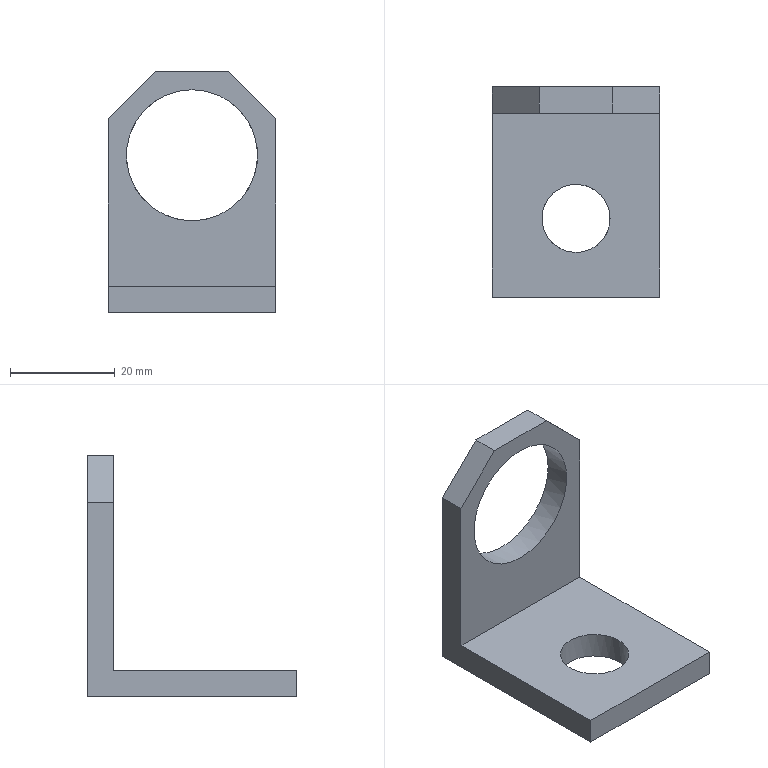Part | NX | features solid 2 | 1 solid | 12 faces | box 32 x 40 x 46 mm | volume 9437 mm3 | plane 10 | cylinder 2 | commonest cylinder face diameters 13 x1 25 x1
STEP:
#1=CARTESIAN_POINT('',(-610.,535.,-367.5));
#2=VERTEX_POINT('',#1);
#3=CARTESIAN_POINT('',(-610.,535.,-380.));
#4=DIRECTION('',(0.,-1.,0.));
#5=DIRECTION('',(0.,0.,1.));
#6=AXIS2_PLACEMENT_3D('',#3,#4,#5);
#7=CIRCLE('',#6,12.5);
#8=EDGE_CURVE('',#2,#2,#7,.T.);
#9=ORIENTED_EDGE('',*,*,#8,.F.);
#10=EDGE_LOOP('',(#9));
#11=FACE_BOUND('',#10,.T.);
#12=CARTESIAN_POINT('',(-594.,535.,-405.));
#13=VERTEX_POINT('',#12);
#14=CARTESIAN_POINT('',(-594.,535.,-373.));
#15=VERTEX_POINT('',#14);
#16=CARTESIAN_POINT('',(-594.,535.,-410.));
#17=DIRECTION('',(0.,0.,1.));
#18=VECTOR('',#17,1000.);
#19=LINE('',#16,#18);
#20=EDGE_CURVE('',#13,#15,#19,.T.);
#21=ORIENTED_EDGE('',*,*,#20,.T.);
#22=CARTESIAN_POINT('',(-603.,535.,-364.));
#23=VERTEX_POINT('',#22);
#24=CARTESIAN_POINT('',(-598.5,535.,-368.5));
#25=DIRECTION('',(0.7071,0.,-0.7071));
#26=VECTOR('',#25,1000.);
#27=LINE('',#24,#26);
#28=EDGE_CURVE('',#15,#23,#27,.F.);
#29=ORIENTED_EDGE('',*,*,#28,.T.);
#30=CARTESIAN_POINT('',(-617.,535.,-364.));
#31=VERTEX_POINT('',#30);
#32=CARTESIAN_POINT('',(-594.,535.,-364.));
#33=DIRECTION('',(-1.,0.,0.));
#34=VECTOR('',#33,1000.);
#35=LINE('',#32,#34);
#36=EDGE_CURVE('',#23,#31,#35,.T.);
#37=ORIENTED_EDGE('',*,*,#36,.T.);
#38=CARTESIAN_POINT('',(-626.,535.,-373.));
#39=VERTEX_POINT('',#38);
#40=CARTESIAN_POINT('',(-605.5,535.,-352.5));
#41=DIRECTION('',(0.7071,0.,0.7071));
#42=VECTOR('',#41,1000.);
#43=LINE('',#40,#42);
#44=EDGE_CURVE('',#31,#39,#43,.F.);
#45=ORIENTED_EDGE('',*,*,#44,.T.);
#46=CARTESIAN_POINT('',(-626.,535.,-405.));
#47=VERTEX_POINT('',#46);
#48=CARTESIAN_POINT('',(-626.,535.,-364.));
#49=DIRECTION('',(0.,0.,-1.));
#50=VECTOR('',#49,1000.);
#51=LINE('',#48,#50);
#52=EDGE_CURVE('',#39,#47,#51,.T.);
#53=ORIENTED_EDGE('',*,*,#52,.T.);
#54=CARTESIAN_POINT('',(-594.,535.,-405.));
#55=DIRECTION('',(1.,0.,0.));
#56=VECTOR('',#55,1000.);
#57=LINE('',#54,#56);
#58=EDGE_CURVE('',#47,#13,#57,.T.);
#59=ORIENTED_EDGE('',*,*,#58,.T.);
#60=EDGE_LOOP('',(#21,#29,#37,#45,#53,#59));
#61=FACE_BOUND('',#60,.T.);
#62=CARTESIAN_POINT('',(-594.,535.,-364.));
#63=DIRECTION('',(0.,-1.,0.));
#64=DIRECTION('',(1.,0.,0.));
#65=AXIS2_PLACEMENT_3D('',#62,#63,#64);
#66=PLANE('',#65);
#67=ADVANCED_FACE('',(#11,#61),#66,.T.);
#68=CARTESIAN_POINT('',(-594.,500.,-410.));
#69=VERTEX_POINT('',#68);
#70=CARTESIAN_POINT('',(-594.,500.,-405.));
#71=VERTEX_POINT('',#70);
#72=CARTESIAN_POINT('',(-594.,500.,-410.));
#73=DIRECTION('',(0.,0.,1.));
#74=VECTOR('',#73,1000.);
#75=LINE('',#72,#74);
#76=EDGE_CURVE('',#69,#71,#75,.T.);
#77=ORIENTED_EDGE('',*,*,#76,.F.);
#78=CARTESIAN_POINT('',(-594.,540.,-410.));
#79=VERTEX_POINT('',#78);
#80=CARTESIAN_POINT('',(-594.,534.,-410.));
#81=DIRECTION('',(0.,1.,0.));
#82=VECTOR('',#81,1000.);
#83=LINE('',#80,#82);
#84=EDGE_CURVE('',#69,#79,#83,.T.);
#85=ORIENTED_EDGE('',*,*,#84,.T.);
#86=CARTESIAN_POINT('',(-594.,540.,-373.));
#87=VERTEX_POINT('',#86);
#88=CARTESIAN_POINT('',(-594.,540.,-410.));
#89=DIRECTION('',(0.,0.,1.));
#90=VECTOR('',#89,1000.);
#91=LINE('',#88,#90);
#92=EDGE_CURVE('',#79,#87,#91,.T.);
#93=ORIENTED_EDGE('',*,*,#92,.T.);
#94=CARTESIAN_POINT('',(-594.,534.,-373.));
#95=DIRECTION('',(0.,-1.,0.));
#96=VECTOR('',#95,1000.);
#97=LINE('',#94,#96);
#98=EDGE_CURVE('',#87,#15,#97,.T.);
#99=ORIENTED_EDGE('',*,*,#98,.T.);
#100=ORIENTED_EDGE('',*,*,#20,.F.);
#101=CARTESIAN_POINT('',(-594.,500.,-405.));
#102=DIRECTION('',(0.,1.,0.));
#103=VECTOR('',#102,1000.);
#104=LINE('',#101,#103);
#105=EDGE_CURVE('',#71,#13,#104,.T.);
#106=ORIENTED_EDGE('',*,*,#105,.F.);
#107=EDGE_LOOP('',(#77,#85,#93,#99,#100,#106));
#108=FACE_BOUND('',#107,.T.);
#109=CARTESIAN_POINT('',(-594.,534.,-410.));
#110=DIRECTION('',(-1.,0.,0.));
#111=DIRECTION('',(0.,0.,-1.));
#112=AXIS2_PLACEMENT_3D('',#109,#110,#111);
#113=PLANE('',#112);
#114=ADVANCED_FACE('',(#108),#113,.F.);
#115=ORIENTED_EDGE('',*,*,#36,.F.);
#116=CARTESIAN_POINT('',(-603.,540.,-364.));
#117=VERTEX_POINT('',#116);
#118=CARTESIAN_POINT('',(-603.,534.,-364.));
#119=DIRECTION('',(0.,1.,0.));
#120=VECTOR('',#119,1000.);
#121=LINE('',#118,#120);
#122=EDGE_CURVE('',#23,#117,#121,.T.);
#123=ORIENTED_EDGE('',*,*,#122,.T.);
#124=CARTESIAN_POINT('',(-617.,540.,-364.));
#125=VERTEX_POINT('',#124);
#126=CARTESIAN_POINT('',(-594.,540.,-364.));
#127=DIRECTION('',(-1.,0.,0.));
#128=VECTOR('',#127,1000.);
#129=LINE('',#126,#128);
#130=EDGE_CURVE('',#117,#125,#129,.T.);
#131=ORIENTED_EDGE('',*,*,#130,.T.);
#132=CARTESIAN_POINT('',(-617.,534.,-364.));
#133=DIRECTION('',(0.,-1.,0.));
#134=VECTOR('',#133,1000.);
#135=LINE('',#132,#134);
#136=EDGE_CURVE('',#125,#31,#135,.T.);
#137=ORIENTED_EDGE('',*,*,#136,.T.);
#138=EDGE_LOOP('',(#115,#123,#131,#137));
#139=FACE_BOUND('',#138,.T.);
#140=CARTESIAN_POINT('',(-594.,534.,-364.));
#141=DIRECTION('',(0.,0.,-1.));
#142=DIRECTION('',(0.,1.,0.));
#143=AXIS2_PLACEMENT_3D('',#140,#141,#142);
#144=PLANE('',#143);
#145=ADVANCED_FACE('',(#139),#144,.F.);
#146=CARTESIAN_POINT('',(-626.,500.,-410.));
#147=VERTEX_POINT('',#146);
#148=CARTESIAN_POINT('',(-626.,540.,-410.));
#149=VERTEX_POINT('',#148);
#150=CARTESIAN_POINT('',(-626.,534.,-410.));
#151=DIRECTION('',(0.,1.,0.));
#152=VECTOR('',#151,1000.);
#153=LINE('',#150,#152);
#154=EDGE_CURVE('',#147,#149,#153,.T.);
#155=ORIENTED_EDGE('',*,*,#154,.F.);
#156=CARTESIAN_POINT('',(-626.,500.,-405.));
#157=VERTEX_POINT('',#156);
#158=CARTESIAN_POINT('',(-626.,500.,-410.));
#159=DIRECTION('',(0.,0.,1.));
#160=VECTOR('',#159,1000.);
#161=LINE('',#158,#160);
#162=EDGE_CURVE('',#147,#157,#161,.T.);
#163=ORIENTED_EDGE('',*,*,#162,.T.);
#164=CARTESIAN_POINT('',(-626.,534.,-405.));
#165=DIRECTION('',(0.,1.,0.));
#166=VECTOR('',#165,1000.);
#167=LINE('',#164,#166);
#168=EDGE_CURVE('',#157,#47,#167,.T.);
#169=ORIENTED_EDGE('',*,*,#168,.T.);
#170=ORIENTED_EDGE('',*,*,#52,.F.);
#171=CARTESIAN_POINT('',(-626.,540.,-373.));
#172=VERTEX_POINT('',#171);
#173=CARTESIAN_POINT('',(-626.,534.,-373.));
#174=DIRECTION('',(0.,1.,0.));
#175=VECTOR('',#174,1000.);
#176=LINE('',#173,#175);
#177=EDGE_CURVE('',#39,#172,#176,.T.);
#178=ORIENTED_EDGE('',*,*,#177,.T.);
#179=CARTESIAN_POINT('',(-626.,540.,-364.));
#180=DIRECTION('',(0.,0.,-1.));
#181=VECTOR('',#180,1000.);
#182=LINE('',#179,#181);
#183=EDGE_CURVE('',#172,#149,#182,.T.);
#184=ORIENTED_EDGE('',*,*,#183,.T.);
#185=EDGE_LOOP('',(#155,#163,#169,#170,#178,#184));
#186=FACE_BOUND('',#185,.T.);
#187=CARTESIAN_POINT('',(-626.,534.,-364.));
#188=DIRECTION('',(1.,0.,0.));
#189=DIRECTION('',(0.,0.,1.));
#190=AXIS2_PLACEMENT_3D('',#187,#188,#189);
#191=PLANE('',#190);
#192=ADVANCED_FACE('',(#186),#191,.F.);
#193=ORIENTED_EDGE('',*,*,#8,.T.);
#194=EDGE_LOOP('',(#193));
#195=FACE_BOUND('',#194,.T.);
#196=CARTESIAN_POINT('',(-597.5,540.,-380.));
#197=VERTEX_POINT('',#196);
#198=CARTESIAN_POINT('',(-610.,540.,-380.));
#199=DIRECTION('',(0.,-1.,0.));
#200=DIRECTION('',(1.,0.,0.));
#201=AXIS2_PLACEMENT_3D('',#198,#199,#200);
#202=CIRCLE('',#201,12.5);
#203=EDGE_CURVE('',#197,#197,#202,.T.);
#204=ORIENTED_EDGE('',*,*,#203,.F.);
#205=EDGE_LOOP('',(#204));
#206=FACE_BOUND('',#205,.T.);
#207=CARTESIAN_POINT('',(-610.,534.,-380.));
#208=DIRECTION('',(0.,1.,0.));
#209=DIRECTION('',(-1.,0.,0.));
#210=AXIS2_PLACEMENT_3D('',#207,#208,#209);
#211=CYLINDRICAL_SURFACE('',#210,12.5);
#212=ADVANCED_FACE('',(#195,#206),#211,.F.);
#213=CARTESIAN_POINT('',(-610.,508.5,-410.));
#214=VERTEX_POINT('',#213);
#215=CARTESIAN_POINT('',(-610.,515.,-410.));
#216=DIRECTION('',(0.,0.,1.));
#217=DIRECTION('',(0.,-1.,0.));
#218=AXIS2_PLACEMENT_3D('',#215,#216,#217);
#219=CIRCLE('',#218,6.5);
#220=EDGE_CURVE('',#214,#214,#219,.T.);
#221=ORIENTED_EDGE('',*,*,#220,.T.);
#222=EDGE_LOOP('',(#221));
#223=FACE_BOUND('',#222,.T.);
#224=ORIENTED_EDGE('',*,*,#84,.F.);
#225=CARTESIAN_POINT('',(-626.,500.,-410.));
#226=DIRECTION('',(1.,0.,0.));
#227=VECTOR('',#226,1000.);
#228=LINE('',#225,#227);
#229=EDGE_CURVE('',#147,#69,#228,.T.);
#230=ORIENTED_EDGE('',*,*,#229,.F.);
#231=ORIENTED_EDGE('',*,*,#154,.T.);
#232=CARTESIAN_POINT('',(-626.,540.,-410.));
#233=DIRECTION('',(1.,0.,0.));
#234=VECTOR('',#233,1000.);
#235=LINE('',#232,#234);
#236=EDGE_CURVE('',#149,#79,#235,.T.);
#237=ORIENTED_EDGE('',*,*,#236,.T.);
#238=EDGE_LOOP('',(#224,#230,#231,#237));
#239=FACE_BOUND('',#238,.T.);
#240=CARTESIAN_POINT('',(-626.,534.,-410.));
#241=DIRECTION('',(0.,0.,1.));
#242=DIRECTION('',(0.,-1.,0.));
#243=AXIS2_PLACEMENT_3D('',#240,#241,#242);
#244=PLANE('',#243);
#245=ADVANCED_FACE('',(#223,#239),#244,.F.);
#246=ORIENTED_EDGE('',*,*,#130,.F.);
#247=CARTESIAN_POINT('',(-603.,540.,-364.));
#248=DIRECTION('',(-0.7071,0.,0.7071));
#249=VECTOR('',#248,1000.);
#250=LINE('',#247,#249);
#251=EDGE_CURVE('',#117,#87,#250,.F.);
#252=ORIENTED_EDGE('',*,*,#251,.T.);
#253=ORIENTED_EDGE('',*,*,#92,.F.);
#254=ORIENTED_EDGE('',*,*,#236,.F.);
#255=ORIENTED_EDGE('',*,*,#183,.F.);
#256=CARTESIAN_POINT('',(-626.,540.,-373.));
#257=DIRECTION('',(-0.7071,0.,-0.7071));
#258=VECTOR('',#257,1000.);
#259=LINE('',#256,#258);
#260=EDGE_CURVE('',#172,#125,#259,.F.);
#261=ORIENTED_EDGE('',*,*,#260,.T.);
#262=EDGE_LOOP('',(#246,#252,#253,#254,#255,#261));
#263=FACE_BOUND('',#262,.T.);
#264=ORIENTED_EDGE('',*,*,#203,.T.);
#265=EDGE_LOOP('',(#264));
#266=FACE_BOUND('',#265,.T.);
#267=CARTESIAN_POINT('',(-594.,540.,-364.));
#268=DIRECTION('',(0.,-1.,0.));
#269=DIRECTION('',(1.,0.,0.));
#270=AXIS2_PLACEMENT_3D('',#267,#268,#269);
#271=PLANE('',#270);
#272=ADVANCED_FACE('',(#263,#266),#271,.F.);
#273=CARTESIAN_POINT('',(-603.5,515.,-405.));
#274=VERTEX_POINT('',#273);
#275=CARTESIAN_POINT('',(-610.,515.,-405.));
#276=DIRECTION('',(0.,0.,-1.));
#277=DIRECTION('',(1.,0.,0.));
#278=AXIS2_PLACEMENT_3D('',#275,#276,#277);
#279=CIRCLE('',#278,6.5);
#280=EDGE_CURVE('',#274,#274,#279,.T.);
#281=ORIENTED_EDGE('',*,*,#280,.T.);
#282=EDGE_LOOP('',(#281));
#283=FACE_BOUND('',#282,.T.);
#284=ORIENTED_EDGE('',*,*,#168,.F.);
#285=CARTESIAN_POINT('',(-594.,500.,-405.));
#286=DIRECTION('',(-1.,0.,0.));
#287=VECTOR('',#286,1000.);
#288=LINE('',#285,#287);
#289=EDGE_CURVE('',#71,#157,#288,.T.);
#290=ORIENTED_EDGE('',*,*,#289,.F.);
#291=ORIENTED_EDGE('',*,*,#105,.T.);
#292=ORIENTED_EDGE('',*,*,#58,.F.);
#293=EDGE_LOOP('',(#284,#290,#291,#292));
#294=FACE_BOUND('',#293,.T.);
#295=CARTESIAN_POINT('',(-594.,500.,-405.));
#296=DIRECTION('',(0.,0.,-1.));
#297=DIRECTION('',(0.,1.,0.));
#298=AXIS2_PLACEMENT_3D('',#295,#296,#297);
#299=PLANE('',#298);
#300=ADVANCED_FACE('',(#283,#294),#299,.F.);
#301=ORIENTED_EDGE('',*,*,#162,.F.);
#302=ORIENTED_EDGE('',*,*,#229,.T.);
#303=ORIENTED_EDGE('',*,*,#76,.T.);
#304=ORIENTED_EDGE('',*,*,#289,.T.);
#305=EDGE_LOOP('',(#301,#302,#303,#304));
#306=FACE_BOUND('',#305,.T.);
#307=CARTESIAN_POINT('',(-594.,500.,-410.));
#308=DIRECTION('',(0.,-1.,0.));
#309=DIRECTION('',(1.,0.,0.));
#310=AXIS2_PLACEMENT_3D('',#307,#308,#309);
#311=PLANE('',#310);
#312=ADVANCED_FACE('',(#306),#311,.T.);
#313=ORIENTED_EDGE('',*,*,#220,.F.);
#314=EDGE_LOOP('',(#313));
#315=FACE_BOUND('',#314,.T.);
#316=ORIENTED_EDGE('',*,*,#280,.F.);
#317=EDGE_LOOP('',(#316));
#318=FACE_BOUND('',#317,.T.);
#319=CARTESIAN_POINT('',(-610.,515.,-410.));
#320=DIRECTION('',(0.,0.,1.));
#321=DIRECTION('',(0.,-1.,0.));
#322=AXIS2_PLACEMENT_3D('',#319,#320,#321);
#323=CYLINDRICAL_SURFACE('',#322,6.5);
#324=ADVANCED_FACE('',(#315,#318),#323,.F.);
#325=ORIENTED_EDGE('',*,*,#28,.F.);
#326=ORIENTED_EDGE('',*,*,#98,.F.);
#327=ORIENTED_EDGE('',*,*,#251,.F.);
#328=ORIENTED_EDGE('',*,*,#122,.F.);
#329=EDGE_LOOP('',(#325,#326,#327,#328));
#330=FACE_BOUND('',#329,.T.);
#331=CARTESIAN_POINT('',(-603.,534.,-364.));
#332=DIRECTION('',(-0.7071,0.,-0.7071));
#333=DIRECTION('',(0.7071,0.,-0.7071));
#334=AXIS2_PLACEMENT_3D('',#331,#332,#333);
#335=PLANE('',#334);
#336=ADVANCED_FACE('',(#330),#335,.F.);
#337=ORIENTED_EDGE('',*,*,#44,.F.);
#338=ORIENTED_EDGE('',*,*,#136,.F.);
#339=ORIENTED_EDGE('',*,*,#260,.F.);
#340=ORIENTED_EDGE('',*,*,#177,.F.);
#341=EDGE_LOOP('',(#337,#338,#339,#340));
#342=FACE_BOUND('',#341,.T.);
#343=CARTESIAN_POINT('',(-626.,534.,-373.));
#344=DIRECTION('',(0.7071,0.,-0.7071));
#345=DIRECTION('',(0.7071,0.,0.7071));
#346=AXIS2_PLACEMENT_3D('',#343,#344,#345);
#347=PLANE('',#346);
#348=ADVANCED_FACE('',(#342),#347,.F.);
#349=CLOSED_SHELL('',(#67,#114,#145,#192,#212,#245,#272,#300,#312,#324,#336,#348));
#350=MANIFOLD_SOLID_BREP('',#349);
#351=(LENGTH_UNIT()NAMED_UNIT(*)SI_UNIT(.MILLI.,.METRE.));
#352=UNCERTAINTY_MEASURE_WITH_UNIT(LENGTH_MEASURE(0.00001),#351,'','');
#353=(NAMED_UNIT(*)PLANE_ANGLE_UNIT()SI_UNIT($,.RADIAN.));
#354=(NAMED_UNIT(*)SI_UNIT($,.STERADIAN.)SOLID_ANGLE_UNIT());
#355=(GEOMETRIC_REPRESENTATION_CONTEXT(3)GLOBAL_UNCERTAINTY_ASSIGNED_CONTEXT((#352))GLOBAL_UNIT_ASSIGNED_CONTEXT((#351,#353,#354))REPRESENTATION_CONTEXT('',''));
#356=ADVANCED_BREP_SHAPE_REPRESENTATION('',(#350),#355);